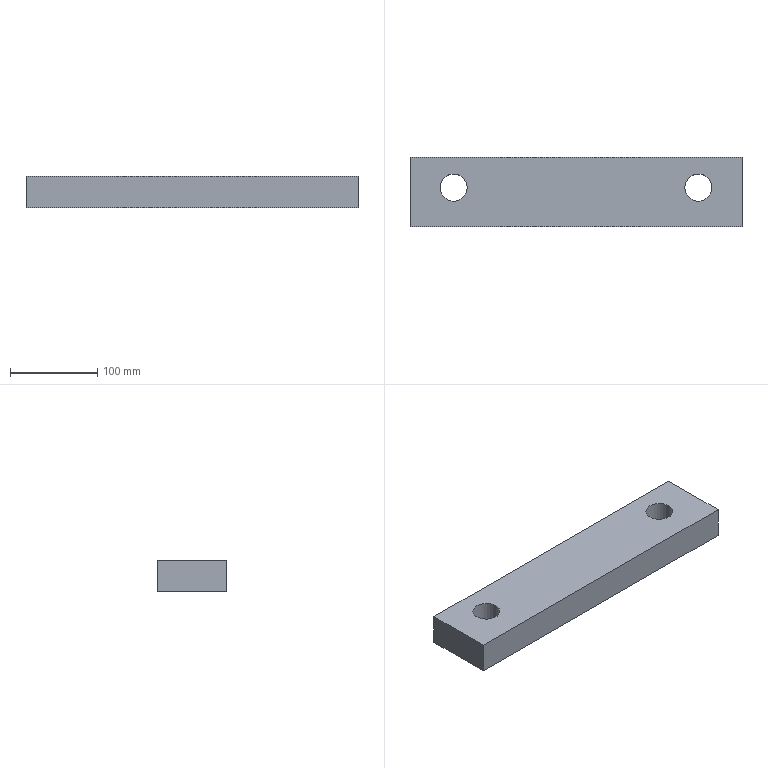Part | SolidWorks | features Extrusion 1, HoleWzd 1 | 1 solid | 10 faces | box 380 x 80 x 36 mm | volume 1040206 mm3 | plane 6 | cylinder 4 | commonest cylinder face diameters 30.958 x4
STEP:
#1=CARTESIAN_POINT('',(-155.479,5.,-18.));
#2=VERTEX_POINT('',#1);
#3=CARTESIAN_POINT('',(-124.521,5.,-18.));
#4=VERTEX_POINT('',#3);
#5=CARTESIAN_POINT('',(-140.,5.,-18.));
#6=DIRECTION('',(0.,0.,1.));
#7=DIRECTION('',(1.,0.,0.));
#8=AXIS2_PLACEMENT_3D('',#5,#6,#7);
#9=CIRCLE('',#8,15.479);
#10=EDGE_CURVE('',#2,#4,#9,.T.);
#11=ORIENTED_EDGE('',*,*,#10,.F.);
#12=CARTESIAN_POINT('',(-155.479,5.,18.));
#13=VERTEX_POINT('',#12);
#14=CARTESIAN_POINT('',(-155.479,5.,18.));
#15=DIRECTION('',(0.,0.,1.));
#16=VECTOR('',#15,1000.);
#17=LINE('',#14,#16);
#18=EDGE_CURVE('',#2,#13,#17,.T.);
#19=ORIENTED_EDGE('',*,*,#18,.T.);
#20=CARTESIAN_POINT('',(-124.521,5.,18.));
#21=VERTEX_POINT('',#20);
#22=CARTESIAN_POINT('',(-140.,5.,18.));
#23=DIRECTION('',(0.,0.,1.));
#24=DIRECTION('',(1.,0.,0.));
#25=AXIS2_PLACEMENT_3D('',#22,#23,#24);
#26=CIRCLE('',#25,15.479);
#27=EDGE_CURVE('',#13,#21,#26,.T.);
#28=ORIENTED_EDGE('',*,*,#27,.T.);
#29=CARTESIAN_POINT('',(-124.521,5.,18.));
#30=DIRECTION('',(0.,0.,1.));
#31=VECTOR('',#30,1000.);
#32=LINE('',#29,#31);
#33=EDGE_CURVE('',#4,#21,#32,.T.);
#34=ORIENTED_EDGE('',*,*,#33,.F.);
#35=EDGE_LOOP('',(#11,#19,#28,#34));
#36=FACE_OUTER_BOUND('',#35,.T.);
#37=CARTESIAN_POINT('',(-140.,5.,18.));
#38=DIRECTION('',(0.,0.,1.));
#39=DIRECTION('',(1.,0.,0.));
#40=AXIS2_PLACEMENT_3D('',#37,#38,#39);
#41=CYLINDRICAL_SURFACE('',#40,15.479);
#42=ADVANCED_FACE('',(#36),#41,.F.);
#43=CARTESIAN_POINT('',(124.521,5.,-18.));
#44=VERTEX_POINT('',#43);
#45=CARTESIAN_POINT('',(155.479,5.,-18.));
#46=VERTEX_POINT('',#45);
#47=CARTESIAN_POINT('',(140.,5.,-18.));
#48=DIRECTION('',(0.,0.,1.));
#49=DIRECTION('',(1.,0.,0.));
#50=AXIS2_PLACEMENT_3D('',#47,#48,#49);
#51=CIRCLE('',#50,15.479);
#52=EDGE_CURVE('',#44,#46,#51,.T.);
#53=ORIENTED_EDGE('',*,*,#52,.F.);
#54=CARTESIAN_POINT('',(124.521,5.,18.));
#55=VERTEX_POINT('',#54);
#56=CARTESIAN_POINT('',(124.521,5.,18.));
#57=DIRECTION('',(0.,0.,1.));
#58=VECTOR('',#57,1000.);
#59=LINE('',#56,#58);
#60=EDGE_CURVE('',#44,#55,#59,.T.);
#61=ORIENTED_EDGE('',*,*,#60,.T.);
#62=CARTESIAN_POINT('',(155.479,5.,18.));
#63=VERTEX_POINT('',#62);
#64=CARTESIAN_POINT('',(140.,5.,18.));
#65=DIRECTION('',(0.,0.,1.));
#66=DIRECTION('',(1.,0.,0.));
#67=AXIS2_PLACEMENT_3D('',#64,#65,#66);
#68=CIRCLE('',#67,15.479);
#69=EDGE_CURVE('',#55,#63,#68,.T.);
#70=ORIENTED_EDGE('',*,*,#69,.T.);
#71=CARTESIAN_POINT('',(155.479,5.,18.));
#72=DIRECTION('',(0.,0.,1.));
#73=VECTOR('',#72,1000.);
#74=LINE('',#71,#73);
#75=EDGE_CURVE('',#46,#63,#74,.T.);
#76=ORIENTED_EDGE('',*,*,#75,.F.);
#77=EDGE_LOOP('',(#53,#61,#70,#76));
#78=FACE_OUTER_BOUND('',#77,.T.);
#79=CARTESIAN_POINT('',(140.,5.,18.));
#80=DIRECTION('',(0.,0.,1.));
#81=DIRECTION('',(1.,0.,0.));
#82=AXIS2_PLACEMENT_3D('',#79,#80,#81);
#83=CYLINDRICAL_SURFACE('',#82,15.479);
#84=ADVANCED_FACE('',(#78),#83,.F.);
#85=CARTESIAN_POINT('',(-190.,40.,-18.));
#86=VERTEX_POINT('',#85);
#87=CARTESIAN_POINT('',(-190.,-40.,-18.));
#88=VERTEX_POINT('',#87);
#89=CARTESIAN_POINT('',(-190.,40.,-18.));
#90=DIRECTION('',(0.,-1.,0.));
#91=VECTOR('',#90,1000.);
#92=LINE('',#89,#91);
#93=EDGE_CURVE('',#86,#88,#92,.T.);
#94=ORIENTED_EDGE('',*,*,#93,.T.);
#95=CARTESIAN_POINT('',(-190.,-40.,18.));
#96=VERTEX_POINT('',#95);
#97=CARTESIAN_POINT('',(-190.,-40.,18.));
#98=DIRECTION('',(0.,0.,-1.));
#99=VECTOR('',#98,1000.);
#100=LINE('',#97,#99);
#101=EDGE_CURVE('',#96,#88,#100,.T.);
#102=ORIENTED_EDGE('',*,*,#101,.F.);
#103=CARTESIAN_POINT('',(-190.,40.,18.));
#104=VERTEX_POINT('',#103);
#105=CARTESIAN_POINT('',(-190.,40.,18.));
#106=DIRECTION('',(0.,-1.,0.));
#107=VECTOR('',#106,1000.);
#108=LINE('',#105,#107);
#109=EDGE_CURVE('',#104,#96,#108,.T.);
#110=ORIENTED_EDGE('',*,*,#109,.F.);
#111=CARTESIAN_POINT('',(-190.,40.,18.));
#112=DIRECTION('',(0.,0.,-1.));
#113=VECTOR('',#112,1000.);
#114=LINE('',#111,#113);
#115=EDGE_CURVE('',#104,#86,#114,.T.);
#116=ORIENTED_EDGE('',*,*,#115,.T.);
#117=EDGE_LOOP('',(#94,#102,#110,#116));
#118=FACE_OUTER_BOUND('',#117,.T.);
#119=CARTESIAN_POINT('',(-190.,40.,18.));
#120=DIRECTION('',(1.,0.,0.));
#121=DIRECTION('',(0.,1.,0.));
#122=AXIS2_PLACEMENT_3D('',#119,#120,#121);
#123=PLANE('',#122);
#124=ADVANCED_FACE('',(#118),#123,.F.);
#125=CARTESIAN_POINT('',(190.,-40.,-18.));
#126=VERTEX_POINT('',#125);
#127=CARTESIAN_POINT('',(-190.,-40.,-18.));
#128=DIRECTION('',(1.,0.,0.));
#129=VECTOR('',#128,1000.);
#130=LINE('',#127,#129);
#131=EDGE_CURVE('',#88,#126,#130,.T.);
#132=ORIENTED_EDGE('',*,*,#131,.T.);
#133=CARTESIAN_POINT('',(190.,-40.,18.));
#134=VERTEX_POINT('',#133);
#135=CARTESIAN_POINT('',(190.,-40.,18.));
#136=DIRECTION('',(0.,0.,-1.));
#137=VECTOR('',#136,1000.);
#138=LINE('',#135,#137);
#139=EDGE_CURVE('',#134,#126,#138,.T.);
#140=ORIENTED_EDGE('',*,*,#139,.F.);
#141=CARTESIAN_POINT('',(-190.,-40.,18.));
#142=DIRECTION('',(1.,0.,0.));
#143=VECTOR('',#142,1000.);
#144=LINE('',#141,#143);
#145=EDGE_CURVE('',#96,#134,#144,.T.);
#146=ORIENTED_EDGE('',*,*,#145,.F.);
#147=ORIENTED_EDGE('',*,*,#101,.T.);
#148=EDGE_LOOP('',(#132,#140,#146,#147));
#149=FACE_OUTER_BOUND('',#148,.T.);
#150=CARTESIAN_POINT('',(-190.,-40.,18.));
#151=DIRECTION('',(0.,1.,0.));
#152=DIRECTION('',(0.,0.,1.));
#153=AXIS2_PLACEMENT_3D('',#150,#151,#152);
#154=PLANE('',#153);
#155=ADVANCED_FACE('',(#149),#154,.F.);
#156=CARTESIAN_POINT('',(190.,40.,-18.));
#157=VERTEX_POINT('',#156);
#158=CARTESIAN_POINT('',(190.,40.,-18.));
#159=DIRECTION('',(0.,1.,0.));
#160=VECTOR('',#159,1000.);
#161=LINE('',#158,#160);
#162=EDGE_CURVE('',#126,#157,#161,.T.);
#163=ORIENTED_EDGE('',*,*,#162,.T.);
#164=CARTESIAN_POINT('',(190.,40.,18.));
#165=VERTEX_POINT('',#164);
#166=CARTESIAN_POINT('',(190.,40.,18.));
#167=DIRECTION('',(0.,0.,-1.));
#168=VECTOR('',#167,1000.);
#169=LINE('',#166,#168);
#170=EDGE_CURVE('',#165,#157,#169,.T.);
#171=ORIENTED_EDGE('',*,*,#170,.F.);
#172=CARTESIAN_POINT('',(190.,40.,18.));
#173=DIRECTION('',(0.,1.,0.));
#174=VECTOR('',#173,1000.);
#175=LINE('',#172,#174);
#176=EDGE_CURVE('',#134,#165,#175,.T.);
#177=ORIENTED_EDGE('',*,*,#176,.F.);
#178=ORIENTED_EDGE('',*,*,#139,.T.);
#179=EDGE_LOOP('',(#163,#171,#177,#178));
#180=FACE_OUTER_BOUND('',#179,.T.);
#181=CARTESIAN_POINT('',(190.,40.,18.));
#182=DIRECTION('',(-1.,0.,0.));
#183=DIRECTION('',(0.,0.,1.));
#184=AXIS2_PLACEMENT_3D('',#181,#182,#183);
#185=PLANE('',#184);
#186=ADVANCED_FACE('',(#180),#185,.F.);
#187=CARTESIAN_POINT('',(-190.,40.,-18.));
#188=DIRECTION('',(-1.,0.,0.));
#189=VECTOR('',#188,1000.);
#190=LINE('',#187,#189);
#191=EDGE_CURVE('',#157,#86,#190,.T.);
#192=ORIENTED_EDGE('',*,*,#191,.T.);
#193=ORIENTED_EDGE('',*,*,#115,.F.);
#194=CARTESIAN_POINT('',(-190.,40.,18.));
#195=DIRECTION('',(-1.,0.,0.));
#196=VECTOR('',#195,1000.);
#197=LINE('',#194,#196);
#198=EDGE_CURVE('',#165,#104,#197,.T.);
#199=ORIENTED_EDGE('',*,*,#198,.F.);
#200=ORIENTED_EDGE('',*,*,#170,.T.);
#201=EDGE_LOOP('',(#192,#193,#199,#200));
#202=FACE_OUTER_BOUND('',#201,.T.);
#203=CARTESIAN_POINT('',(-190.,40.,18.));
#204=DIRECTION('',(0.,-1.,0.));
#205=DIRECTION('',(1.,0.,0.));
#206=AXIS2_PLACEMENT_3D('',#203,#204,#205);
#207=PLANE('',#206);
#208=ADVANCED_FACE('',(#202),#207,.F.);
#209=CARTESIAN_POINT('',(-140.,5.,18.));
#210=DIRECTION('',(0.,0.,1.));
#211=DIRECTION('',(1.,0.,0.));
#212=AXIS2_PLACEMENT_3D('',#209,#210,#211);
#213=CIRCLE('',#212,15.479);
#214=EDGE_CURVE('',#21,#13,#213,.T.);
#215=ORIENTED_EDGE('',*,*,#214,.F.);
#216=ORIENTED_EDGE('',*,*,#27,.F.);
#217=EDGE_LOOP('',(#215,#216));
#218=FACE_BOUND('',#217,.T.);
#219=CARTESIAN_POINT('',(140.,5.,18.));
#220=DIRECTION('',(0.,0.,1.));
#221=DIRECTION('',(1.,0.,0.));
#222=AXIS2_PLACEMENT_3D('',#219,#220,#221);
#223=CIRCLE('',#222,15.479);
#224=EDGE_CURVE('',#63,#55,#223,.T.);
#225=ORIENTED_EDGE('',*,*,#224,.F.);
#226=ORIENTED_EDGE('',*,*,#69,.F.);
#227=EDGE_LOOP('',(#225,#226));
#228=FACE_BOUND('',#227,.T.);
#229=ORIENTED_EDGE('',*,*,#109,.T.);
#230=ORIENTED_EDGE('',*,*,#145,.T.);
#231=ORIENTED_EDGE('',*,*,#176,.T.);
#232=ORIENTED_EDGE('',*,*,#198,.T.);
#233=EDGE_LOOP('',(#229,#230,#231,#232));
#234=FACE_OUTER_BOUND('',#233,.T.);
#235=CARTESIAN_POINT('',(-190.,-40.,18.));
#236=DIRECTION('',(0.,0.,1.));
#237=DIRECTION('',(1.,0.,0.));
#238=AXIS2_PLACEMENT_3D('',#235,#236,#237);
#239=PLANE('',#238);
#240=ADVANCED_FACE('',(#218,#228,#234),#239,.T.);
#241=CARTESIAN_POINT('',(-140.,5.,-18.));
#242=DIRECTION('',(0.,0.,1.));
#243=DIRECTION('',(1.,0.,0.));
#244=AXIS2_PLACEMENT_3D('',#241,#242,#243);
#245=CIRCLE('',#244,15.479);
#246=EDGE_CURVE('',#4,#2,#245,.T.);
#247=ORIENTED_EDGE('',*,*,#246,.T.);
#248=ORIENTED_EDGE('',*,*,#10,.T.);
#249=EDGE_LOOP('',(#247,#248));
#250=FACE_BOUND('',#249,.T.);
#251=CARTESIAN_POINT('',(140.,5.,-18.));
#252=DIRECTION('',(0.,0.,1.));
#253=DIRECTION('',(1.,0.,0.));
#254=AXIS2_PLACEMENT_3D('',#251,#252,#253);
#255=CIRCLE('',#254,15.479);
#256=EDGE_CURVE('',#46,#44,#255,.T.);
#257=ORIENTED_EDGE('',*,*,#256,.T.);
#258=ORIENTED_EDGE('',*,*,#52,.T.);
#259=EDGE_LOOP('',(#257,#258));
#260=FACE_BOUND('',#259,.T.);
#261=ORIENTED_EDGE('',*,*,#93,.F.);
#262=ORIENTED_EDGE('',*,*,#191,.F.);
#263=ORIENTED_EDGE('',*,*,#162,.F.);
#264=ORIENTED_EDGE('',*,*,#131,.F.);
#265=EDGE_LOOP('',(#261,#262,#263,#264));
#266=FACE_OUTER_BOUND('',#265,.T.);
#267=CARTESIAN_POINT('',(-190.,-40.,-18.));
#268=DIRECTION('',(0.,0.,1.));
#269=DIRECTION('',(1.,0.,0.));
#270=AXIS2_PLACEMENT_3D('',#267,#268,#269);
#271=PLANE('',#270);
#272=ADVANCED_FACE('',(#250,#260,#266),#271,.F.);
#273=ORIENTED_EDGE('',*,*,#60,.F.);
#274=ORIENTED_EDGE('',*,*,#256,.F.);
#275=ORIENTED_EDGE('',*,*,#75,.T.);
#276=ORIENTED_EDGE('',*,*,#224,.T.);
#277=EDGE_LOOP('',(#273,#274,#275,#276));
#278=FACE_OUTER_BOUND('',#277,.T.);
#279=CARTESIAN_POINT('',(140.,5.,18.));
#280=DIRECTION('',(0.,0.,1.));
#281=DIRECTION('',(1.,0.,0.));
#282=AXIS2_PLACEMENT_3D('',#279,#280,#281);
#283=CYLINDRICAL_SURFACE('',#282,15.479);
#284=ADVANCED_FACE('',(#278),#283,.F.);
#285=ORIENTED_EDGE('',*,*,#18,.F.);
#286=ORIENTED_EDGE('',*,*,#246,.F.);
#287=ORIENTED_EDGE('',*,*,#33,.T.);
#288=ORIENTED_EDGE('',*,*,#214,.T.);
#289=EDGE_LOOP('',(#285,#286,#287,#288));
#290=FACE_OUTER_BOUND('',#289,.T.);
#291=CARTESIAN_POINT('',(-140.,5.,18.));
#292=DIRECTION('',(0.,0.,1.));
#293=DIRECTION('',(1.,0.,0.));
#294=AXIS2_PLACEMENT_3D('',#291,#292,#293);
#295=CYLINDRICAL_SURFACE('',#294,15.479);
#296=ADVANCED_FACE('',(#290),#295,.F.);
#297=CLOSED_SHELL('',(#42,#84,#124,#155,#186,#208,#240,#272,#284,#296));
#298=MANIFOLD_SOLID_BREP('',#297);
#299=CARTESIAN_POINT('',(0.,0.,0.));
#300=DIRECTION('',(0.,0.,1.));
#301=DIRECTION('',(1.,0.,0.));
#302=AXIS2_PLACEMENT_3D('',#299,#300,#301);
#303=(LENGTH_UNIT()NAMED_UNIT(*)SI_UNIT(.MILLI.,.METRE.));
#304=UNCERTAINTY_MEASURE_WITH_UNIT(LENGTH_MEASURE(0.00001),#303,'','');
#305=(NAMED_UNIT(*)PLANE_ANGLE_UNIT()SI_UNIT($,.RADIAN.));
#306=(NAMED_UNIT(*)SI_UNIT($,.STERADIAN.)SOLID_ANGLE_UNIT());
#307=(GEOMETRIC_REPRESENTATION_CONTEXT(3)GLOBAL_UNCERTAINTY_ASSIGNED_CONTEXT((#304))GLOBAL_UNIT_ASSIGNED_CONTEXT((#303,#305,#306))REPRESENTATION_CONTEXT('',''));
#308=ADVANCED_BREP_SHAPE_REPRESENTATION('',(#298,#302),#307);